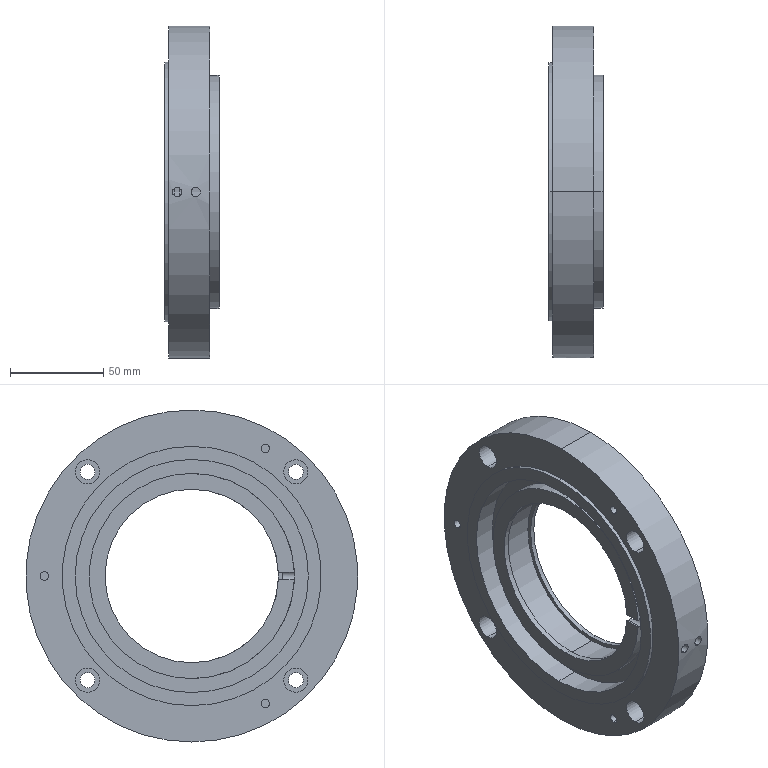Part | STEP file | 46 Spindle Front Sleeve 2 | 1 solid | 70 faces | box 29 x 178 x 178 mm | volume 367063 mm3 | cylinder 52 | plane 18 | commonest cylinder face diameters 8 x8 13 x8 5 x7 4.5 x6 93 x5 125 x4